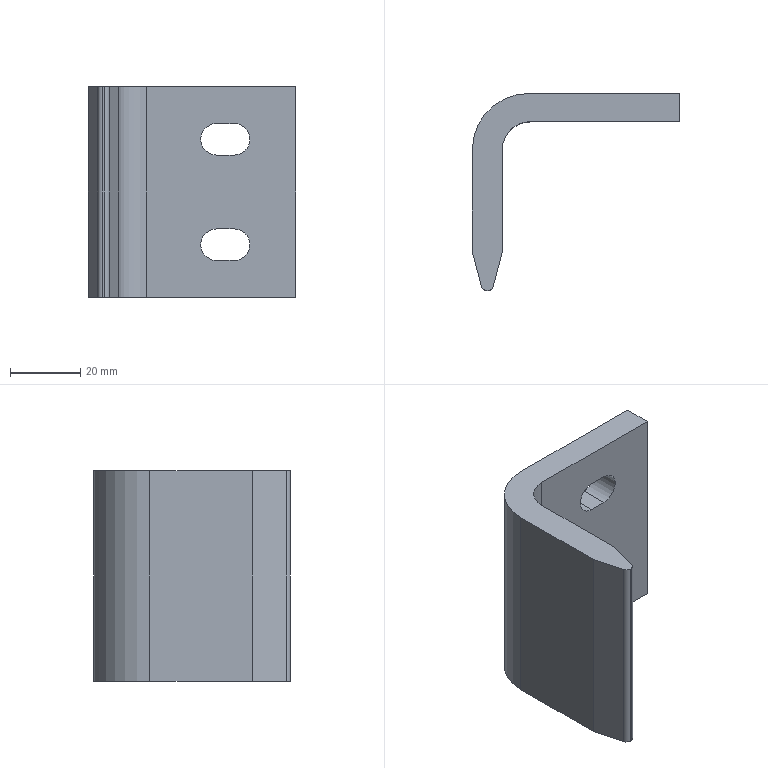Part | SolidWorks | features BaseBody 1 | 1 solid | 22 faces | box 59 x 56 x 60 mm | volume 46684 mm3 | plane 14 | cylinder 8 | commonest cylinder face diameters 9 x4 3 x2 16 x1 32 x1
STEP:
#1=CARTESIAN_POINT('',(701.696,-3638.473,1021.471));
#2=VERTEX_POINT('',#1);
#3=CARTESIAN_POINT('',(658.696,-3638.473,1021.471));
#4=VERTEX_POINT('',#3);
#5=CARTESIAN_POINT('',(701.696,-3638.473,1021.471));
#6=DIRECTION('',(-1.,0.,0.));
#7=VECTOR('',#6,1000.);
#8=LINE('',#5,#7);
#9=EDGE_CURVE('',#2,#4,#8,.T.);
#10=ORIENTED_EDGE('',*,*,#9,.T.);
#11=CARTESIAN_POINT('',(658.696,-3638.473,1081.471));
#12=VERTEX_POINT('',#11);
#13=CARTESIAN_POINT('',(658.696,-3638.473,1021.471));
#14=DIRECTION('',(0.,0.,1.));
#15=VECTOR('',#14,1000.);
#16=LINE('',#13,#15);
#17=EDGE_CURVE('',#4,#12,#16,.T.);
#18=ORIENTED_EDGE('',*,*,#17,.T.);
#19=CARTESIAN_POINT('',(701.696,-3638.473,1081.471));
#20=VERTEX_POINT('',#19);
#21=CARTESIAN_POINT('',(701.696,-3638.473,1081.471));
#22=DIRECTION('',(1.,0.,0.));
#23=VECTOR('',#22,1000.);
#24=LINE('',#21,#23);
#25=EDGE_CURVE('',#12,#20,#24,.T.);
#26=ORIENTED_EDGE('',*,*,#25,.T.);
#27=CARTESIAN_POINT('',(701.696,-3638.473,1021.471));
#28=DIRECTION('',(0.,0.,-1.));
#29=VECTOR('',#28,1000.);
#30=LINE('',#27,#29);
#31=EDGE_CURVE('',#20,#2,#30,.T.);
#32=ORIENTED_EDGE('',*,*,#31,.T.);
#33=EDGE_LOOP('',(#10,#18,#26,#32));
#34=FACE_OUTER_BOUND('',#33,.T.);
#35=CARTESIAN_POINT('',(679.196,-3638.473,1070.971));
#36=VERTEX_POINT('',#35);
#37=CARTESIAN_POINT('',(679.196,-3638.473,1061.971));
#38=VERTEX_POINT('',#37);
#39=CARTESIAN_POINT('',(679.196,-3638.473,1066.471));
#40=DIRECTION('',(0.,-1.,0.));
#41=DIRECTION('',(0.,0.,1.));
#42=AXIS2_PLACEMENT_3D('',#39,#40,#41);
#43=CIRCLE('',#42,4.5);
#44=EDGE_CURVE('',#36,#38,#43,.T.);
#45=ORIENTED_EDGE('',*,*,#44,.T.);
#46=CARTESIAN_POINT('',(684.196,-3638.473,1061.971));
#47=VERTEX_POINT('',#46);
#48=CARTESIAN_POINT('',(701.696,-3638.473,1061.971));
#49=DIRECTION('',(1.,0.,0.));
#50=VECTOR('',#49,1000.);
#51=LINE('',#48,#50);
#52=EDGE_CURVE('',#38,#47,#51,.T.);
#53=ORIENTED_EDGE('',*,*,#52,.T.);
#54=CARTESIAN_POINT('',(684.196,-3638.473,1070.971));
#55=VERTEX_POINT('',#54);
#56=CARTESIAN_POINT('',(684.196,-3638.473,1066.471));
#57=DIRECTION('',(0.,-1.,0.));
#58=DIRECTION('',(0.,0.,1.));
#59=AXIS2_PLACEMENT_3D('',#56,#57,#58);
#60=CIRCLE('',#59,4.5);
#61=EDGE_CURVE('',#47,#55,#60,.T.);
#62=ORIENTED_EDGE('',*,*,#61,.T.);
#63=CARTESIAN_POINT('',(701.696,-3638.473,1070.971));
#64=DIRECTION('',(-1.,0.,0.));
#65=VECTOR('',#64,1000.);
#66=LINE('',#63,#65);
#67=EDGE_CURVE('',#55,#36,#66,.T.);
#68=ORIENTED_EDGE('',*,*,#67,.T.);
#69=EDGE_LOOP('',(#45,#53,#62,#68));
#70=FACE_BOUND('',#69,.T.);
#71=CARTESIAN_POINT('',(679.196,-3638.473,1040.971));
#72=VERTEX_POINT('',#71);
#73=CARTESIAN_POINT('',(679.196,-3638.473,1031.971));
#74=VERTEX_POINT('',#73);
#75=CARTESIAN_POINT('',(679.196,-3638.473,1036.471));
#76=DIRECTION('',(0.,-1.,0.));
#77=DIRECTION('',(0.,0.,-1.));
#78=AXIS2_PLACEMENT_3D('',#75,#76,#77);
#79=CIRCLE('',#78,4.5);
#80=EDGE_CURVE('',#72,#74,#79,.T.);
#81=ORIENTED_EDGE('',*,*,#80,.T.);
#82=CARTESIAN_POINT('',(684.196,-3638.473,1031.971));
#83=VERTEX_POINT('',#82);
#84=CARTESIAN_POINT('',(701.696,-3638.473,1031.971));
#85=DIRECTION('',(1.,0.,0.));
#86=VECTOR('',#85,1000.);
#87=LINE('',#84,#86);
#88=EDGE_CURVE('',#74,#83,#87,.T.);
#89=ORIENTED_EDGE('',*,*,#88,.T.);
#90=CARTESIAN_POINT('',(684.196,-3638.473,1040.971));
#91=VERTEX_POINT('',#90);
#92=CARTESIAN_POINT('',(684.196,-3638.473,1036.471));
#93=DIRECTION('',(0.,-1.,0.));
#94=DIRECTION('',(0.,0.,-1.));
#95=AXIS2_PLACEMENT_3D('',#92,#93,#94);
#96=CIRCLE('',#95,4.5);
#97=EDGE_CURVE('',#83,#91,#96,.T.);
#98=ORIENTED_EDGE('',*,*,#97,.T.);
#99=CARTESIAN_POINT('',(701.696,-3638.473,1040.971));
#100=DIRECTION('',(-1.,0.,0.));
#101=VECTOR('',#100,1000.);
#102=LINE('',#99,#101);
#103=EDGE_CURVE('',#91,#72,#102,.T.);
#104=ORIENTED_EDGE('',*,*,#103,.T.);
#105=EDGE_LOOP('',(#81,#89,#98,#104));
#106=FACE_BOUND('',#105,.T.);
#107=CARTESIAN_POINT('',(701.696,-3638.473,1021.471));
#108=DIRECTION('',(0.,1.,0.));
#109=DIRECTION('',(0.,0.,1.));
#110=AXIS2_PLACEMENT_3D('',#107,#108,#109);
#111=PLANE('',#110);
#112=ADVANCED_FACE('',(#34,#70,#106),#111,.T.);
#113=CARTESIAN_POINT('',(642.696,-3654.473,1021.471));
#114=VERTEX_POINT('',#113);
#115=CARTESIAN_POINT('',(658.696,-3654.473,1021.471));
#116=DIRECTION('',(0.,0.,1.));
#117=DIRECTION('',(-1.,0.,0.));
#118=AXIS2_PLACEMENT_3D('',#115,#116,#117);
#119=CIRCLE('',#118,16.);
#120=EDGE_CURVE('',#4,#114,#119,.T.);
#121=ORIENTED_EDGE('',*,*,#120,.T.);
#122=CARTESIAN_POINT('',(642.696,-3654.473,1081.471));
#123=VERTEX_POINT('',#122);
#124=CARTESIAN_POINT('',(642.696,-3654.473,1021.471));
#125=DIRECTION('',(0.,0.,1.));
#126=VECTOR('',#125,1000.);
#127=LINE('',#124,#126);
#128=EDGE_CURVE('',#114,#123,#127,.T.);
#129=ORIENTED_EDGE('',*,*,#128,.T.);
#130=CARTESIAN_POINT('',(658.696,-3654.473,1081.471));
#131=DIRECTION('',(0.,0.,-1.));
#132=DIRECTION('',(-1.,0.,0.));
#133=AXIS2_PLACEMENT_3D('',#130,#131,#132);
#134=CIRCLE('',#133,16.);
#135=EDGE_CURVE('',#123,#12,#134,.T.);
#136=ORIENTED_EDGE('',*,*,#135,.T.);
#137=ORIENTED_EDGE('',*,*,#17,.F.);
#138=EDGE_LOOP('',(#121,#129,#136,#137));
#139=FACE_OUTER_BOUND('',#138,.T.);
#140=CARTESIAN_POINT('',(658.696,-3654.473,1021.471));
#141=DIRECTION('',(0.,0.,-1.));
#142=DIRECTION('',(-1.,0.,0.));
#143=AXIS2_PLACEMENT_3D('',#140,#141,#142);
#144=CYLINDRICAL_SURFACE('',#143,16.);
#145=ADVANCED_FACE('',(#139),#144,.T.);
#146=CARTESIAN_POINT('',(659.196,-3646.473,1021.471));
#147=VERTEX_POINT('',#146);
#148=CARTESIAN_POINT('',(701.696,-3646.473,1021.471));
#149=VERTEX_POINT('',#148);
#150=CARTESIAN_POINT('',(662.963,-3646.473,1021.471));
#151=DIRECTION('',(1.,0.,0.));
#152=VECTOR('',#151,1000.);
#153=LINE('',#150,#152);
#154=EDGE_CURVE('',#147,#149,#153,.T.);
#155=ORIENTED_EDGE('',*,*,#154,.F.);
#156=CARTESIAN_POINT('',(651.196,-3654.473,1021.471));
#157=VERTEX_POINT('',#156);
#158=CARTESIAN_POINT('',(659.196,-3654.473,1021.471));
#159=DIRECTION('',(0.,0.,-1.));
#160=DIRECTION('',(-1.,0.,0.));
#161=AXIS2_PLACEMENT_3D('',#158,#159,#160);
#162=CIRCLE('',#161,8.);
#163=EDGE_CURVE('',#157,#147,#162,.T.);
#164=ORIENTED_EDGE('',*,*,#163,.F.);
#165=CARTESIAN_POINT('',(651.196,-3683.673,1021.471));
#166=VERTEX_POINT('',#165);
#167=CARTESIAN_POINT('',(651.196,-3655.736,1021.471));
#168=DIRECTION('',(0.,1.,0.));
#169=VECTOR('',#168,1000.);
#170=LINE('',#167,#169);
#171=EDGE_CURVE('',#166,#157,#170,.T.);
#172=ORIENTED_EDGE('',*,*,#171,.F.);
#173=CARTESIAN_POINT('',(648.6,-3693.361,1021.471));
#174=VERTEX_POINT('',#173);
#175=CARTESIAN_POINT('',(648.6,-3693.361,1021.471));
#176=DIRECTION('',(0.2588,0.9659,0.));
#177=VECTOR('',#176,1000.);
#178=LINE('',#175,#177);
#179=EDGE_CURVE('',#174,#166,#178,.T.);
#180=ORIENTED_EDGE('',*,*,#179,.F.);
#181=CARTESIAN_POINT('',(647.151,-3694.473,1021.471));
#182=VERTEX_POINT('',#181);
#183=CARTESIAN_POINT('',(647.151,-3692.973,1021.471));
#184=DIRECTION('',(0.,0.,1.));
#185=DIRECTION('',(-1.,0.,0.));
#186=AXIS2_PLACEMENT_3D('',#183,#184,#185);
#187=CIRCLE('',#186,1.5);
#188=EDGE_CURVE('',#182,#174,#187,.T.);
#189=ORIENTED_EDGE('',*,*,#188,.F.);
#190=CARTESIAN_POINT('',(646.74,-3694.473,1021.471));
#191=VERTEX_POINT('',#190);
#192=CARTESIAN_POINT('',(646.74,-3694.473,1021.471));
#193=DIRECTION('',(1.,0.,0.));
#194=VECTOR('',#193,1000.);
#195=LINE('',#192,#194);
#196=EDGE_CURVE('',#191,#182,#195,.T.);
#197=ORIENTED_EDGE('',*,*,#196,.F.);
#198=CARTESIAN_POINT('',(645.291,-3693.361,1021.471));
#199=VERTEX_POINT('',#198);
#200=CARTESIAN_POINT('',(646.74,-3692.973,1021.471));
#201=DIRECTION('',(0.,0.,1.));
#202=DIRECTION('',(-1.,0.,0.));
#203=AXIS2_PLACEMENT_3D('',#200,#201,#202);
#204=CIRCLE('',#203,1.5);
#205=EDGE_CURVE('',#199,#191,#204,.T.);
#206=ORIENTED_EDGE('',*,*,#205,.F.);
#207=CARTESIAN_POINT('',(642.696,-3683.673,1021.471));
#208=VERTEX_POINT('',#207);
#209=CARTESIAN_POINT('',(642.696,-3683.673,1021.471));
#210=DIRECTION('',(0.2588,-0.9659,0.));
#211=VECTOR('',#210,1000.);
#212=LINE('',#209,#211);
#213=EDGE_CURVE('',#208,#199,#212,.T.);
#214=ORIENTED_EDGE('',*,*,#213,.F.);
#215=CARTESIAN_POINT('',(642.696,-3655.736,1021.471));
#216=DIRECTION('',(0.,-1.,0.));
#217=VECTOR('',#216,1000.);
#218=LINE('',#215,#217);
#219=EDGE_CURVE('',#114,#208,#218,.T.);
#220=ORIENTED_EDGE('',*,*,#219,.F.);
#221=ORIENTED_EDGE('',*,*,#120,.F.);
#222=ORIENTED_EDGE('',*,*,#9,.F.);
#223=CARTESIAN_POINT('',(701.696,-3655.736,1021.471));
#224=DIRECTION('',(0.,1.,0.));
#225=VECTOR('',#224,1000.);
#226=LINE('',#223,#225);
#227=EDGE_CURVE('',#149,#2,#226,.T.);
#228=ORIENTED_EDGE('',*,*,#227,.F.);
#229=EDGE_LOOP('',(#155,#164,#172,#180,#189,#197,#206,#214,#220,#221,#222,#228));
#230=FACE_OUTER_BOUND('',#229,.T.);
#231=CARTESIAN_POINT('',(662.963,-3655.736,1021.471));
#232=DIRECTION('',(0.,0.,1.));
#233=DIRECTION('',(1.,0.,0.));
#234=AXIS2_PLACEMENT_3D('',#231,#232,#233);
#235=PLANE('',#234);
#236=ADVANCED_FACE('',(#230),#235,.F.);
#237=ORIENTED_EDGE('',*,*,#227,.T.);
#238=ORIENTED_EDGE('',*,*,#31,.F.);
#239=CARTESIAN_POINT('',(701.696,-3646.473,1081.471));
#240=VERTEX_POINT('',#239);
#241=CARTESIAN_POINT('',(701.696,-3646.473,1081.471));
#242=DIRECTION('',(0.,-1.,0.));
#243=VECTOR('',#242,1000.);
#244=LINE('',#241,#243);
#245=EDGE_CURVE('',#20,#240,#244,.T.);
#246=ORIENTED_EDGE('',*,*,#245,.T.);
#247=CARTESIAN_POINT('',(701.696,-3646.473,1021.471));
#248=DIRECTION('',(0.,0.,-1.));
#249=VECTOR('',#248,1000.);
#250=LINE('',#247,#249);
#251=EDGE_CURVE('',#240,#149,#250,.T.);
#252=ORIENTED_EDGE('',*,*,#251,.T.);
#253=EDGE_LOOP('',(#237,#238,#246,#252));
#254=FACE_OUTER_BOUND('',#253,.T.);
#255=CARTESIAN_POINT('',(701.696,-3646.473,1021.471));
#256=DIRECTION('',(1.,0.,0.));
#257=DIRECTION('',(0.,1.,0.));
#258=AXIS2_PLACEMENT_3D('',#255,#256,#257);
#259=PLANE('',#258);
#260=ADVANCED_FACE('',(#254),#259,.T.);
#261=CARTESIAN_POINT('',(659.196,-3646.473,1081.471));
#262=VERTEX_POINT('',#261);
#263=CARTESIAN_POINT('',(662.963,-3646.473,1081.471));
#264=DIRECTION('',(1.,0.,0.));
#265=VECTOR('',#264,1000.);
#266=LINE('',#263,#265);
#267=EDGE_CURVE('',#262,#240,#266,.T.);
#268=ORIENTED_EDGE('',*,*,#267,.T.);
#269=ORIENTED_EDGE('',*,*,#245,.F.);
#270=ORIENTED_EDGE('',*,*,#25,.F.);
#271=ORIENTED_EDGE('',*,*,#135,.F.);
#272=CARTESIAN_POINT('',(642.696,-3683.673,1081.471));
#273=VERTEX_POINT('',#272);
#274=CARTESIAN_POINT('',(642.696,-3655.736,1081.471));
#275=DIRECTION('',(0.,-1.,0.));
#276=VECTOR('',#275,1000.);
#277=LINE('',#274,#276);
#278=EDGE_CURVE('',#123,#273,#277,.T.);
#279=ORIENTED_EDGE('',*,*,#278,.T.);
#280=CARTESIAN_POINT('',(645.291,-3693.361,1081.471));
#281=VERTEX_POINT('',#280);
#282=CARTESIAN_POINT('',(642.696,-3683.673,1081.471));
#283=DIRECTION('',(0.2588,-0.9659,0.));
#284=VECTOR('',#283,1000.);
#285=LINE('',#282,#284);
#286=EDGE_CURVE('',#273,#281,#285,.T.);
#287=ORIENTED_EDGE('',*,*,#286,.T.);
#288=CARTESIAN_POINT('',(646.74,-3694.473,1081.471));
#289=VERTEX_POINT('',#288);
#290=CARTESIAN_POINT('',(646.74,-3692.973,1081.471));
#291=DIRECTION('',(0.,0.,1.));
#292=DIRECTION('',(-1.,0.,0.));
#293=AXIS2_PLACEMENT_3D('',#290,#291,#292);
#294=CIRCLE('',#293,1.5);
#295=EDGE_CURVE('',#281,#289,#294,.T.);
#296=ORIENTED_EDGE('',*,*,#295,.T.);
#297=CARTESIAN_POINT('',(647.151,-3694.473,1081.471));
#298=VERTEX_POINT('',#297);
#299=CARTESIAN_POINT('',(646.74,-3694.473,1081.471));
#300=DIRECTION('',(-1.,0.,0.));
#301=VECTOR('',#300,1000.);
#302=LINE('',#299,#301);
#303=EDGE_CURVE('',#298,#289,#302,.T.);
#304=ORIENTED_EDGE('',*,*,#303,.F.);
#305=CARTESIAN_POINT('',(648.6,-3693.361,1081.471));
#306=VERTEX_POINT('',#305);
#307=CARTESIAN_POINT('',(647.151,-3692.973,1081.471));
#308=DIRECTION('',(0.,0.,1.));
#309=DIRECTION('',(-1.,0.,0.));
#310=AXIS2_PLACEMENT_3D('',#307,#308,#309);
#311=CIRCLE('',#310,1.5);
#312=EDGE_CURVE('',#298,#306,#311,.T.);
#313=ORIENTED_EDGE('',*,*,#312,.T.);
#314=CARTESIAN_POINT('',(651.196,-3683.673,1081.471));
#315=VERTEX_POINT('',#314);
#316=CARTESIAN_POINT('',(648.6,-3693.361,1081.471));
#317=DIRECTION('',(0.2588,0.9659,0.));
#318=VECTOR('',#317,1000.);
#319=LINE('',#316,#318);
#320=EDGE_CURVE('',#306,#315,#319,.T.);
#321=ORIENTED_EDGE('',*,*,#320,.T.);
#322=CARTESIAN_POINT('',(651.196,-3654.473,1081.471));
#323=VERTEX_POINT('',#322);
#324=CARTESIAN_POINT('',(651.196,-3655.736,1081.471));
#325=DIRECTION('',(0.,1.,0.));
#326=VECTOR('',#325,1000.);
#327=LINE('',#324,#326);
#328=EDGE_CURVE('',#315,#323,#327,.T.);
#329=ORIENTED_EDGE('',*,*,#328,.T.);
#330=CARTESIAN_POINT('',(659.196,-3654.473,1081.471));
#331=DIRECTION('',(0.,0.,-1.));
#332=DIRECTION('',(-1.,0.,0.));
#333=AXIS2_PLACEMENT_3D('',#330,#331,#332);
#334=CIRCLE('',#333,8.);
#335=EDGE_CURVE('',#323,#262,#334,.T.);
#336=ORIENTED_EDGE('',*,*,#335,.T.);
#337=EDGE_LOOP('',(#268,#269,#270,#271,#279,#287,#296,#304,#313,#321,#329,#336));
#338=FACE_OUTER_BOUND('',#337,.T.);
#339=CARTESIAN_POINT('',(662.963,-3655.736,1081.471));
#340=DIRECTION('',(0.,0.,1.));
#341=DIRECTION('',(1.,0.,0.));
#342=AXIS2_PLACEMENT_3D('',#339,#340,#341);
#343=PLANE('',#342);
#344=ADVANCED_FACE('',(#338),#343,.T.);
#345=CARTESIAN_POINT('',(679.196,-3646.473,1061.971));
#346=VERTEX_POINT('',#345);
#347=CARTESIAN_POINT('',(679.196,-3617.792,1061.971));
#348=DIRECTION('',(0.,1.,0.));
#349=VECTOR('',#348,1000.);
#350=LINE('',#347,#349);
#351=EDGE_CURVE('',#346,#38,#350,.T.);
#352=ORIENTED_EDGE('',*,*,#351,.F.);
#353=CARTESIAN_POINT('',(684.196,-3646.473,1061.971));
#354=VERTEX_POINT('',#353);
#355=CARTESIAN_POINT('',(679.196,-3646.473,1061.971));
#356=DIRECTION('',(-1.,0.,0.));
#357=VECTOR('',#356,1000.);
#358=LINE('',#355,#357);
#359=EDGE_CURVE('',#354,#346,#358,.T.);
#360=ORIENTED_EDGE('',*,*,#359,.F.);
#361=CARTESIAN_POINT('',(684.196,-3617.792,1061.971));
#362=DIRECTION('',(0.,-1.,0.));
#363=VECTOR('',#362,1000.);
#364=LINE('',#361,#363);
#365=EDGE_CURVE('',#47,#354,#364,.T.);
#366=ORIENTED_EDGE('',*,*,#365,.F.);
#367=ORIENTED_EDGE('',*,*,#52,.F.);
#368=EDGE_LOOP('',(#352,#360,#366,#367));
#369=FACE_OUTER_BOUND('',#368,.T.);
#370=CARTESIAN_POINT('',(679.196,-3617.792,1061.971));
#371=DIRECTION('',(0.,0.,-1.));
#372=DIRECTION('',(-1.,0.,0.));
#373=AXIS2_PLACEMENT_3D('',#370,#371,#372);
#374=PLANE('',#373);
#375=ADVANCED_FACE('',(#369),#374,.F.);
#376=CARTESIAN_POINT('',(679.196,-3646.473,1070.971));
#377=VERTEX_POINT('',#376);
#378=CARTESIAN_POINT('',(679.196,-3617.792,1070.971));
#379=DIRECTION('',(0.,1.,0.));
#380=VECTOR('',#379,1000.);
#381=LINE('',#378,#380);
#382=EDGE_CURVE('',#377,#36,#381,.T.);
#383=ORIENTED_EDGE('',*,*,#382,.F.);
#384=CARTESIAN_POINT('',(679.196,-3646.473,1066.471));
#385=DIRECTION('',(0.,1.,0.));
#386=DIRECTION('',(0.,0.,1.));
#387=AXIS2_PLACEMENT_3D('',#384,#385,#386);
#388=CIRCLE('',#387,4.5);
#389=EDGE_CURVE('',#346,#377,#388,.T.);
#390=ORIENTED_EDGE('',*,*,#389,.F.);
#391=ORIENTED_EDGE('',*,*,#351,.T.);
#392=ORIENTED_EDGE('',*,*,#44,.F.);
#393=EDGE_LOOP('',(#383,#390,#391,#392));
#394=FACE_OUTER_BOUND('',#393,.T.);
#395=CARTESIAN_POINT('',(679.196,-3617.792,1066.471));
#396=DIRECTION('',(0.,1.,0.));
#397=DIRECTION('',(0.,0.,1.));
#398=AXIS2_PLACEMENT_3D('',#395,#396,#397);
#399=CYLINDRICAL_SURFACE('',#398,4.5);
#400=ADVANCED_FACE('',(#394),#399,.F.);
#401=CARTESIAN_POINT('',(684.196,-3646.473,1070.971));
#402=VERTEX_POINT('',#401);
#403=CARTESIAN_POINT('',(684.196,-3617.792,1070.971));
#404=DIRECTION('',(0.,1.,0.));
#405=VECTOR('',#404,1000.);
#406=LINE('',#403,#405);
#407=EDGE_CURVE('',#402,#55,#406,.T.);
#408=ORIENTED_EDGE('',*,*,#407,.F.);
#409=CARTESIAN_POINT('',(684.196,-3646.473,1070.971));
#410=DIRECTION('',(1.,0.,0.));
#411=VECTOR('',#410,1000.);
#412=LINE('',#409,#411);
#413=EDGE_CURVE('',#377,#402,#412,.T.);
#414=ORIENTED_EDGE('',*,*,#413,.F.);
#415=ORIENTED_EDGE('',*,*,#382,.T.);
#416=ORIENTED_EDGE('',*,*,#67,.F.);
#417=EDGE_LOOP('',(#408,#414,#415,#416));
#418=FACE_OUTER_BOUND('',#417,.T.);
#419=CARTESIAN_POINT('',(684.196,-3617.792,1070.971));
#420=DIRECTION('',(0.,0.,1.));
#421=DIRECTION('',(1.,0.,0.));
#422=AXIS2_PLACEMENT_3D('',#419,#420,#421);
#423=PLANE('',#422);
#424=ADVANCED_FACE('',(#418),#423,.F.);
#425=ORIENTED_EDGE('',*,*,#365,.T.);
#426=CARTESIAN_POINT('',(684.196,-3646.473,1066.471));
#427=DIRECTION('',(0.,1.,0.));
#428=DIRECTION('',(0.,0.,1.));
#429=AXIS2_PLACEMENT_3D('',#426,#427,#428);
#430=CIRCLE('',#429,4.5);
#431=EDGE_CURVE('',#402,#354,#430,.T.);
#432=ORIENTED_EDGE('',*,*,#431,.F.);
#433=ORIENTED_EDGE('',*,*,#407,.T.);
#434=ORIENTED_EDGE('',*,*,#61,.F.);
#435=EDGE_LOOP('',(#425,#432,#433,#434));
#436=FACE_OUTER_BOUND('',#435,.T.);
#437=CARTESIAN_POINT('',(684.196,-3617.792,1066.471));
#438=DIRECTION('',(0.,1.,0.));
#439=DIRECTION('',(0.,0.,1.));
#440=AXIS2_PLACEMENT_3D('',#437,#438,#439);
#441=CYLINDRICAL_SURFACE('',#440,4.5);
#442=ADVANCED_FACE('',(#436),#441,.F.);
#443=CARTESIAN_POINT('',(679.196,-3646.473,1031.971));
#444=VERTEX_POINT('',#443);
#445=CARTESIAN_POINT('',(679.196,-3617.792,1031.971));
#446=DIRECTION('',(0.,1.,0.));
#447=VECTOR('',#446,1000.);
#448=LINE('',#445,#447);
#449=EDGE_CURVE('',#444,#74,#448,.T.);
#450=ORIENTED_EDGE('',*,*,#449,.F.);
#451=CARTESIAN_POINT('',(684.196,-3646.473,1031.971));
#452=VERTEX_POINT('',#451);
#453=CARTESIAN_POINT('',(684.196,-3646.473,1031.971));
#454=DIRECTION('',(-1.,0.,0.));
#455=VECTOR('',#454,1000.);
#456=LINE('',#453,#455);
#457=EDGE_CURVE('',#452,#444,#456,.T.);
#458=ORIENTED_EDGE('',*,*,#457,.F.);
#459=CARTESIAN_POINT('',(684.196,-3617.792,1031.971));
#460=DIRECTION('',(0.,-1.,0.));
#461=VECTOR('',#460,1000.);
#462=LINE('',#459,#461);
#463=EDGE_CURVE('',#83,#452,#462,.T.);
#464=ORIENTED_EDGE('',*,*,#463,.F.);
#465=ORIENTED_EDGE('',*,*,#88,.F.);
#466=EDGE_LOOP('',(#450,#458,#464,#465));
#467=FACE_OUTER_BOUND('',#466,.T.);
#468=CARTESIAN_POINT('',(684.196,-3617.792,1031.971));
#469=DIRECTION('',(0.,0.,-1.));
#470=DIRECTION('',(-1.,0.,0.));
#471=AXIS2_PLACEMENT_3D('',#468,#469,#470);
#472=PLANE('',#471);
#473=ADVANCED_FACE('',(#467),#472,.F.);
#474=CARTESIAN_POINT('',(679.196,-3646.473,1040.971));
#475=VERTEX_POINT('',#474);
#476=CARTESIAN_POINT('',(679.196,-3617.792,1040.971));
#477=DIRECTION('',(0.,1.,0.));
#478=VECTOR('',#477,1000.);
#479=LINE('',#476,#478);
#480=EDGE_CURVE('',#475,#72,#479,.T.);
#481=ORIENTED_EDGE('',*,*,#480,.F.);
#482=CARTESIAN_POINT('',(679.196,-3646.473,1036.471));
#483=DIRECTION('',(0.,1.,0.));
#484=DIRECTION('',(0.,0.,-1.));
#485=AXIS2_PLACEMENT_3D('',#482,#483,#484);
#486=CIRCLE('',#485,4.5);
#487=EDGE_CURVE('',#444,#475,#486,.T.);
#488=ORIENTED_EDGE('',*,*,#487,.F.);
#489=ORIENTED_EDGE('',*,*,#449,.T.);
#490=ORIENTED_EDGE('',*,*,#80,.F.);
#491=EDGE_LOOP('',(#481,#488,#489,#490));
#492=FACE_OUTER_BOUND('',#491,.T.);
#493=CARTESIAN_POINT('',(679.196,-3617.792,1036.471));
#494=DIRECTION('',(0.,-1.,0.));
#495=DIRECTION('',(0.,0.,-1.));
#496=AXIS2_PLACEMENT_3D('',#493,#494,#495);
#497=CYLINDRICAL_SURFACE('',#496,4.5);
#498=ADVANCED_FACE('',(#492),#497,.F.);
#499=CARTESIAN_POINT('',(684.196,-3646.473,1040.971));
#500=VERTEX_POINT('',#499);
#501=CARTESIAN_POINT('',(684.196,-3617.792,1040.971));
#502=DIRECTION('',(0.,1.,0.));
#503=VECTOR('',#502,1000.);
#504=LINE('',#501,#503);
#505=EDGE_CURVE('',#500,#91,#504,.T.);
#506=ORIENTED_EDGE('',*,*,#505,.F.);
#507=CARTESIAN_POINT('',(679.196,-3646.473,1040.971));
#508=DIRECTION('',(1.,0.,0.));
#509=VECTOR('',#508,1000.);
#510=LINE('',#507,#509);
#511=EDGE_CURVE('',#475,#500,#510,.T.);
#512=ORIENTED_EDGE('',*,*,#511,.F.);
#513=ORIENTED_EDGE('',*,*,#480,.T.);
#514=ORIENTED_EDGE('',*,*,#103,.F.);
#515=EDGE_LOOP('',(#506,#512,#513,#514));
#516=FACE_OUTER_BOUND('',#515,.T.);
#517=CARTESIAN_POINT('',(679.196,-3617.792,1040.971));
#518=DIRECTION('',(0.,0.,1.));
#519=DIRECTION('',(1.,0.,0.));
#520=AXIS2_PLACEMENT_3D('',#517,#518,#519);
#521=PLANE('',#520);
#522=ADVANCED_FACE('',(#516),#521,.F.);
#523=ORIENTED_EDGE('',*,*,#463,.T.);
#524=CARTESIAN_POINT('',(684.196,-3646.473,1036.471));
#525=DIRECTION('',(0.,1.,0.));
#526=DIRECTION('',(0.,0.,-1.));
#527=AXIS2_PLACEMENT_3D('',#524,#525,#526);
#528=CIRCLE('',#527,4.5);
#529=EDGE_CURVE('',#500,#452,#528,.T.);
#530=ORIENTED_EDGE('',*,*,#529,.F.);
#531=ORIENTED_EDGE('',*,*,#505,.T.);
#532=ORIENTED_EDGE('',*,*,#97,.F.);
#533=EDGE_LOOP('',(#523,#530,#531,#532));
#534=FACE_OUTER_BOUND('',#533,.T.);
#535=CARTESIAN_POINT('',(684.196,-3617.792,1036.471));
#536=DIRECTION('',(0.,-1.,0.));
#537=DIRECTION('',(0.,0.,-1.));
#538=AXIS2_PLACEMENT_3D('',#535,#536,#537);
#539=CYLINDRICAL_SURFACE('',#538,4.5);
#540=ADVANCED_FACE('',(#534),#539,.F.);
#541=ORIENTED_EDGE('',*,*,#219,.T.);
#542=CARTESIAN_POINT('',(642.696,-3683.673,1021.471));
#543=DIRECTION('',(0.,0.,1.));
#544=VECTOR('',#543,1000.);
#545=LINE('',#542,#544);
#546=EDGE_CURVE('',#208,#273,#545,.T.);
#547=ORIENTED_EDGE('',*,*,#546,.T.);
#548=ORIENTED_EDGE('',*,*,#278,.F.);
#549=ORIENTED_EDGE('',*,*,#128,.F.);
#550=EDGE_LOOP('',(#541,#547,#548,#549));
#551=FACE_OUTER_BOUND('',#550,.T.);
#552=CARTESIAN_POINT('',(642.696,-3654.473,1021.471));
#553=DIRECTION('',(-1.,0.,0.));
#554=DIRECTION('',(0.,0.,1.));
#555=AXIS2_PLACEMENT_3D('',#552,#553,#554);
#556=PLANE('',#555);
#557=ADVANCED_FACE('',(#551),#556,.T.);
#558=ORIENTED_EDGE('',*,*,#154,.T.);
#559=ORIENTED_EDGE('',*,*,#251,.F.);
#560=ORIENTED_EDGE('',*,*,#267,.F.);
#561=CARTESIAN_POINT('',(659.196,-3646.473,1021.471));
#562=DIRECTION('',(0.,0.,-1.));
#563=VECTOR('',#562,1000.);
#564=LINE('',#561,#563);
#565=EDGE_CURVE('',#262,#147,#564,.T.);
#566=ORIENTED_EDGE('',*,*,#565,.T.);
#567=EDGE_LOOP('',(#558,#559,#560,#566));
#568=FACE_OUTER_BOUND('',#567,.T.);
#569=ORIENTED_EDGE('',*,*,#389,.T.);
#570=ORIENTED_EDGE('',*,*,#413,.T.);
#571=ORIENTED_EDGE('',*,*,#431,.T.);
#572=ORIENTED_EDGE('',*,*,#359,.T.);
#573=EDGE_LOOP('',(#569,#570,#571,#572));
#574=FACE_BOUND('',#573,.T.);
#575=ORIENTED_EDGE('',*,*,#487,.T.);
#576=ORIENTED_EDGE('',*,*,#511,.T.);
#577=ORIENTED_EDGE('',*,*,#529,.T.);
#578=ORIENTED_EDGE('',*,*,#457,.T.);
#579=EDGE_LOOP('',(#575,#576,#577,#578));
#580=FACE_BOUND('',#579,.T.);
#581=CARTESIAN_POINT('',(659.196,-3646.473,1021.471));
#582=DIRECTION('',(0.,-1.,0.));
#583=DIRECTION('',(0.,0.,-1.));
#584=AXIS2_PLACEMENT_3D('',#581,#582,#583);
#585=PLANE('',#584);
#586=ADVANCED_FACE('',(#568,#574,#580),#585,.T.);
#587=ORIENTED_EDGE('',*,*,#163,.T.);
#588=ORIENTED_EDGE('',*,*,#565,.F.);
#589=ORIENTED_EDGE('',*,*,#335,.F.);
#590=CARTESIAN_POINT('',(651.196,-3654.473,1021.471));
#591=DIRECTION('',(0.,0.,-1.));
#592=VECTOR('',#591,1000.);
#593=LINE('',#590,#592);
#594=EDGE_CURVE('',#323,#157,#593,.T.);
#595=ORIENTED_EDGE('',*,*,#594,.T.);
#596=EDGE_LOOP('',(#587,#588,#589,#595));
#597=FACE_OUTER_BOUND('',#596,.T.);
#598=CARTESIAN_POINT('',(659.196,-3654.473,1081.471));
#599=DIRECTION('',(0.,0.,-1.));
#600=DIRECTION('',(-1.,0.,0.));
#601=AXIS2_PLACEMENT_3D('',#598,#599,#600);
#602=CYLINDRICAL_SURFACE('',#601,8.);
#603=ADVANCED_FACE('',(#597),#602,.F.);
#604=ORIENTED_EDGE('',*,*,#171,.T.);
#605=ORIENTED_EDGE('',*,*,#594,.F.);
#606=ORIENTED_EDGE('',*,*,#328,.F.);
#607=CARTESIAN_POINT('',(651.196,-3683.673,1021.471));
#608=DIRECTION('',(0.,0.,-1.));
#609=VECTOR('',#608,1000.);
#610=LINE('',#607,#609);
#611=EDGE_CURVE('',#315,#166,#610,.T.);
#612=ORIENTED_EDGE('',*,*,#611,.T.);
#613=EDGE_LOOP('',(#604,#605,#606,#612));
#614=FACE_OUTER_BOUND('',#613,.T.);
#615=CARTESIAN_POINT('',(651.196,-3683.673,1021.471));
#616=DIRECTION('',(1.,0.,0.));
#617=DIRECTION('',(0.,1.,0.));
#618=AXIS2_PLACEMENT_3D('',#615,#616,#617);
#619=PLANE('',#618);
#620=ADVANCED_FACE('',(#614),#619,.T.);
#621=ORIENTED_EDGE('',*,*,#179,.T.);
#622=ORIENTED_EDGE('',*,*,#611,.F.);
#623=ORIENTED_EDGE('',*,*,#320,.F.);
#624=CARTESIAN_POINT('',(648.6,-3693.361,1021.471));
#625=DIRECTION('',(0.,0.,-1.));
#626=VECTOR('',#625,1000.);
#627=LINE('',#624,#626);
#628=EDGE_CURVE('',#306,#174,#627,.T.);
#629=ORIENTED_EDGE('',*,*,#628,.T.);
#630=EDGE_LOOP('',(#621,#622,#623,#629));
#631=FACE_OUTER_BOUND('',#630,.T.);
#632=CARTESIAN_POINT('',(648.6,-3693.361,1021.471));
#633=DIRECTION('',(0.9659,-0.2588,0.));
#634=DIRECTION('',(0.2588,0.9659,0.));
#635=AXIS2_PLACEMENT_3D('',#632,#633,#634);
#636=PLANE('',#635);
#637=ADVANCED_FACE('',(#631),#636,.T.);
#638=ORIENTED_EDGE('',*,*,#188,.T.);
#639=ORIENTED_EDGE('',*,*,#628,.F.);
#640=ORIENTED_EDGE('',*,*,#312,.F.);
#641=CARTESIAN_POINT('',(647.151,-3694.473,1021.471));
#642=DIRECTION('',(0.,0.,-1.));
#643=VECTOR('',#642,1000.);
#644=LINE('',#641,#643);
#645=EDGE_CURVE('',#298,#182,#644,.T.);
#646=ORIENTED_EDGE('',*,*,#645,.T.);
#647=EDGE_LOOP('',(#638,#639,#640,#646));
#648=FACE_OUTER_BOUND('',#647,.T.);
#649=CARTESIAN_POINT('',(647.151,-3692.973,1021.471));
#650=DIRECTION('',(0.,0.,-1.));
#651=DIRECTION('',(-1.,0.,0.));
#652=AXIS2_PLACEMENT_3D('',#649,#650,#651);
#653=CYLINDRICAL_SURFACE('',#652,1.5);
#654=ADVANCED_FACE('',(#648),#653,.T.);
#655=ORIENTED_EDGE('',*,*,#205,.T.);
#656=CARTESIAN_POINT('',(646.74,-3694.473,1021.471));
#657=DIRECTION('',(0.,0.,1.));
#658=VECTOR('',#657,1000.);
#659=LINE('',#656,#658);
#660=EDGE_CURVE('',#191,#289,#659,.T.);
#661=ORIENTED_EDGE('',*,*,#660,.T.);
#662=ORIENTED_EDGE('',*,*,#295,.F.);
#663=CARTESIAN_POINT('',(645.291,-3693.361,1021.471));
#664=DIRECTION('',(0.,0.,-1.));
#665=VECTOR('',#664,1000.);
#666=LINE('',#663,#665);
#667=EDGE_CURVE('',#281,#199,#666,.T.);
#668=ORIENTED_EDGE('',*,*,#667,.T.);
#669=EDGE_LOOP('',(#655,#661,#662,#668));
#670=FACE_OUTER_BOUND('',#669,.T.);
#671=CARTESIAN_POINT('',(646.74,-3692.973,1021.471));
#672=DIRECTION('',(0.,0.,-1.));
#673=DIRECTION('',(-1.,0.,0.));
#674=AXIS2_PLACEMENT_3D('',#671,#672,#673);
#675=CYLINDRICAL_SURFACE('',#674,1.5);
#676=ADVANCED_FACE('',(#670),#675,.T.);
#677=ORIENTED_EDGE('',*,*,#213,.T.);
#678=ORIENTED_EDGE('',*,*,#667,.F.);
#679=ORIENTED_EDGE('',*,*,#286,.F.);
#680=ORIENTED_EDGE('',*,*,#546,.F.);
#681=EDGE_LOOP('',(#677,#678,#679,#680));
#682=FACE_OUTER_BOUND('',#681,.T.);
#683=CARTESIAN_POINT('',(642.696,-3683.673,1021.471));
#684=DIRECTION('',(-0.9659,-0.2588,0.));
#685=DIRECTION('',(0.2588,-0.9659,0.));
#686=AXIS2_PLACEMENT_3D('',#683,#684,#685);
#687=PLANE('',#686);
#688=ADVANCED_FACE('',(#682),#687,.T.);
#689=ORIENTED_EDGE('',*,*,#196,.T.);
#690=ORIENTED_EDGE('',*,*,#645,.F.);
#691=ORIENTED_EDGE('',*,*,#303,.T.);
#692=ORIENTED_EDGE('',*,*,#660,.F.);
#693=EDGE_LOOP('',(#689,#690,#691,#692));
#694=FACE_OUTER_BOUND('',#693,.T.);
#695=CARTESIAN_POINT('',(646.74,-3694.473,1021.471));
#696=DIRECTION('',(0.,-1.,0.));
#697=DIRECTION('',(0.,0.,-1.));
#698=AXIS2_PLACEMENT_3D('',#695,#696,#697);
#699=PLANE('',#698);
#700=ADVANCED_FACE('',(#694),#699,.T.);
#701=CLOSED_SHELL('',(#112,#145,#236,#260,#344,#375,#400,#424,#442,#473,#498,#522,#540,#557,#586,#603,#620,#637,#654,#676,#688,#700));
#702=MANIFOLD_SOLID_BREP('',#701);
#703=CARTESIAN_POINT('',(0.,0.,0.));
#704=DIRECTION('',(0.,0.,1.));
#705=DIRECTION('',(1.,0.,0.));
#706=AXIS2_PLACEMENT_3D('',#703,#704,#705);
#707=(LENGTH_UNIT()NAMED_UNIT(*)SI_UNIT(.MILLI.,.METRE.));
#708=UNCERTAINTY_MEASURE_WITH_UNIT(LENGTH_MEASURE(0.00001),#707,'','');
#709=(NAMED_UNIT(*)PLANE_ANGLE_UNIT()SI_UNIT($,.RADIAN.));
#710=(NAMED_UNIT(*)SI_UNIT($,.STERADIAN.)SOLID_ANGLE_UNIT());
#711=(GEOMETRIC_REPRESENTATION_CONTEXT(3)GLOBAL_UNCERTAINTY_ASSIGNED_CONTEXT((#708))GLOBAL_UNIT_ASSIGNED_CONTEXT((#707,#709,#710))REPRESENTATION_CONTEXT('',''));
#712=ADVANCED_BREP_SHAPE_REPRESENTATION('',(#702,#706),#711);